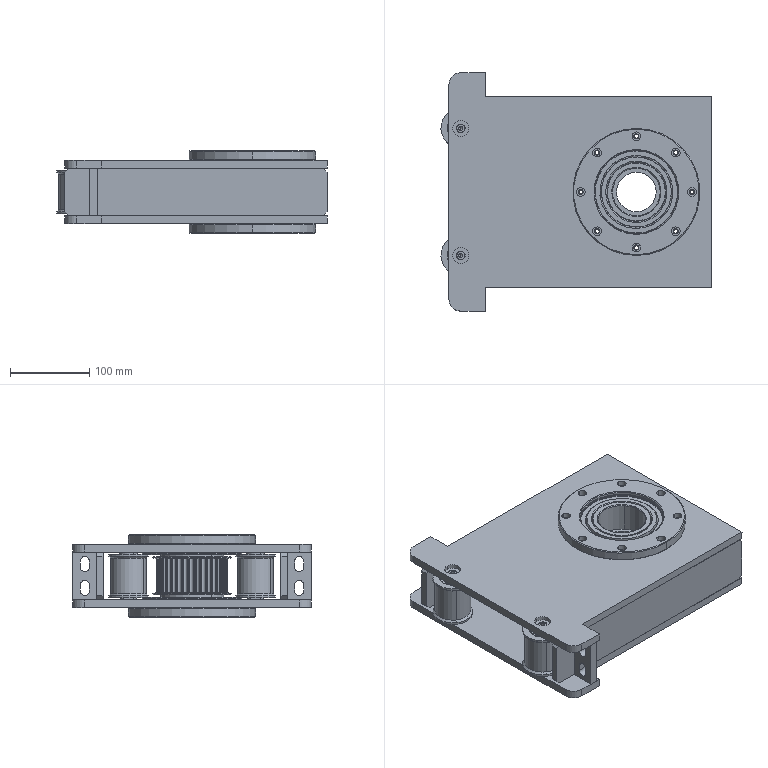Part | SolidWorks | features LocalLPattern 1, ReferencePattern 1 | 22 solids | 1717 faces | box 340 x 300 x 104 mm | volume 2603051 mm3 | cylinder 533 | sphere 440 | plane 374 | torus 270 | cone 100 | commonest cylinder face diameters 1.56 x90 5.14 x53 11 x52 5 x36 90.298 x36 6.6 x32